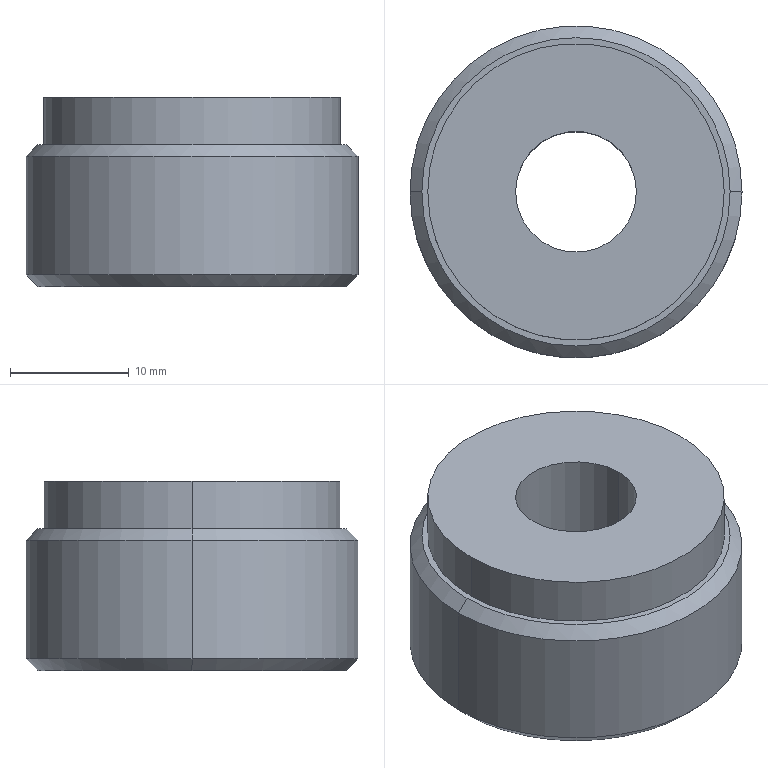Part | STEP file | Screen clamp lock nut 2 | 1 solid | 16 faces | box 28 x 28 x 16 mm | volume 7694 mm3 | cylinder 6 | cone 6 | plane 4 | commonest cylinder face diameters 10.2 x2 25 x2 28 x2
STEP:
#1=CARTESIAN_POINT('',(5.1,0.,1.));
#2=VERTEX_POINT('',#1);
#3=CARTESIAN_POINT('',(-5.1,0.,1.));
#4=VERTEX_POINT('',#3);
#5=CARTESIAN_POINT('',(0.,0.,1.));
#6=DIRECTION('',(0.,0.,-1.));
#7=DIRECTION('',(-1.,0.,0.));
#8=AXIS2_PLACEMENT_3D('',#5,#6,#7);
#9=CIRCLE('',#8,5.1);
#10=EDGE_CURVE('',#2,#4,#9,.T.);
#11=ORIENTED_EDGE('',*,*,#10,.T.);
#12=CARTESIAN_POINT('',(-5.1,0.,16.));
#13=VERTEX_POINT('',#12);
#14=CARTESIAN_POINT('',(-5.1,0.,16.));
#15=DIRECTION('',(0.,0.,1.));
#16=VECTOR('',#15,1000.);
#17=LINE('',#14,#16);
#18=EDGE_CURVE('',#4,#13,#17,.T.);
#19=ORIENTED_EDGE('',*,*,#18,.T.);
#20=CARTESIAN_POINT('',(5.1,0.,16.));
#21=VERTEX_POINT('',#20);
#22=CARTESIAN_POINT('',(0.,0.,16.));
#23=DIRECTION('',(0.,0.,1.));
#24=DIRECTION('',(1.,0.,0.));
#25=AXIS2_PLACEMENT_3D('',#22,#23,#24);
#26=CIRCLE('',#25,5.1);
#27=EDGE_CURVE('',#13,#21,#26,.T.);
#28=ORIENTED_EDGE('',*,*,#27,.T.);
#29=CARTESIAN_POINT('',(5.1,0.,16.));
#30=DIRECTION('',(0.,0.,1.));
#31=VECTOR('',#30,1000.);
#32=LINE('',#29,#31);
#33=EDGE_CURVE('',#2,#21,#32,.T.);
#34=ORIENTED_EDGE('',*,*,#33,.F.);
#35=EDGE_LOOP('',(#11,#19,#28,#34));
#36=FACE_OUTER_BOUND('',#35,.T.);
#37=CARTESIAN_POINT('',(0.,0.,16.));
#38=DIRECTION('',(0.,0.,1.));
#39=DIRECTION('',(1.,0.,0.));
#40=AXIS2_PLACEMENT_3D('',#37,#38,#39);
#41=CYLINDRICAL_SURFACE('',#40,5.1);
#42=ADVANCED_FACE('',(#36),#41,.F.);
#43=CARTESIAN_POINT('',(13.,0.,12.));
#44=VERTEX_POINT('',#43);
#45=CARTESIAN_POINT('',(-13.,0.,12.));
#46=VERTEX_POINT('',#45);
#47=CARTESIAN_POINT('',(0.,0.,12.));
#48=DIRECTION('',(0.,0.,1.));
#49=DIRECTION('',(1.,0.,0.));
#50=AXIS2_PLACEMENT_3D('',#47,#48,#49);
#51=CIRCLE('',#50,13.);
#52=EDGE_CURVE('',#44,#46,#51,.T.);
#53=ORIENTED_EDGE('',*,*,#52,.F.);
#54=CARTESIAN_POINT('',(14.,0.,11.));
#55=VERTEX_POINT('',#54);
#56=CARTESIAN_POINT('',(13.,0.,12.));
#57=DIRECTION('',(0.7071,0.,-0.7071));
#58=VECTOR('',#57,1000.);
#59=LINE('',#56,#58);
#60=EDGE_CURVE('',#44,#55,#59,.T.);
#61=ORIENTED_EDGE('',*,*,#60,.T.);
#62=CARTESIAN_POINT('',(-14.,0.,11.));
#63=VERTEX_POINT('',#62);
#64=CARTESIAN_POINT('',(0.,0.,11.));
#65=DIRECTION('',(0.,0.,-1.));
#66=DIRECTION('',(1.,0.,0.));
#67=AXIS2_PLACEMENT_3D('',#64,#65,#66);
#68=CIRCLE('',#67,14.);
#69=EDGE_CURVE('',#63,#55,#68,.T.);
#70=ORIENTED_EDGE('',*,*,#69,.F.);
#71=CARTESIAN_POINT('',(-13.,0.,12.));
#72=DIRECTION('',(-0.7071,0.,-0.7071));
#73=VECTOR('',#72,1000.);
#74=LINE('',#71,#73);
#75=EDGE_CURVE('',#46,#63,#74,.T.);
#76=ORIENTED_EDGE('',*,*,#75,.F.);
#77=EDGE_LOOP('',(#53,#61,#70,#76));
#78=FACE_OUTER_BOUND('',#77,.T.);
#79=CARTESIAN_POINT('',(0.,0.,12.));
#80=DIRECTION('',(0.,0.,-1.));
#81=DIRECTION('',(-1.,0.,0.));
#82=AXIS2_PLACEMENT_3D('',#79,#80,#81);
#83=CONICAL_SURFACE('',#82,13.,0.7854);
#84=ADVANCED_FACE('',(#78),#83,.T.);
#85=CARTESIAN_POINT('',(-13.,0.,0.));
#86=VERTEX_POINT('',#85);
#87=CARTESIAN_POINT('',(13.,0.,0.));
#88=VERTEX_POINT('',#87);
#89=CARTESIAN_POINT('',(0.,0.,0.));
#90=DIRECTION('',(0.,0.,-1.));
#91=DIRECTION('',(1.,0.,0.));
#92=AXIS2_PLACEMENT_3D('',#89,#90,#91);
#93=CIRCLE('',#92,13.);
#94=EDGE_CURVE('',#86,#88,#93,.T.);
#95=ORIENTED_EDGE('',*,*,#94,.F.);
#96=CARTESIAN_POINT('',(-14.,0.,1.));
#97=VERTEX_POINT('',#96);
#98=CARTESIAN_POINT('',(-14.,0.,1.));
#99=DIRECTION('',(-0.7071,0.,0.7071));
#100=VECTOR('',#99,1000.);
#101=LINE('',#98,#100);
#102=EDGE_CURVE('',#86,#97,#101,.T.);
#103=ORIENTED_EDGE('',*,*,#102,.T.);
#104=CARTESIAN_POINT('',(14.,0.,1.));
#105=VERTEX_POINT('',#104);
#106=CARTESIAN_POINT('',(0.,0.,1.));
#107=DIRECTION('',(0.,0.,1.));
#108=DIRECTION('',(1.,0.,0.));
#109=AXIS2_PLACEMENT_3D('',#106,#107,#108);
#110=CIRCLE('',#109,14.);
#111=EDGE_CURVE('',#105,#97,#110,.T.);
#112=ORIENTED_EDGE('',*,*,#111,.F.);
#113=CARTESIAN_POINT('',(14.,0.,1.));
#114=DIRECTION('',(0.7071,0.,0.7071));
#115=VECTOR('',#114,1000.);
#116=LINE('',#113,#115);
#117=EDGE_CURVE('',#88,#105,#116,.T.);
#118=ORIENTED_EDGE('',*,*,#117,.F.);
#119=EDGE_LOOP('',(#95,#103,#112,#118));
#120=FACE_OUTER_BOUND('',#119,.T.);
#121=CARTESIAN_POINT('',(0.,0.,1.));
#122=DIRECTION('',(0.,0.,1.));
#123=DIRECTION('',(1.,0.,0.));
#124=AXIS2_PLACEMENT_3D('',#121,#122,#123);
#125=CONICAL_SURFACE('',#124,14.,0.7854);
#126=ADVANCED_FACE('',(#120),#125,.T.);
#127=CARTESIAN_POINT('',(10.,0.,1.));
#128=VERTEX_POINT('',#127);
#129=CARTESIAN_POINT('',(-10.,0.,1.));
#130=VERTEX_POINT('',#129);
#131=CARTESIAN_POINT('',(0.,0.,1.));
#132=DIRECTION('',(0.,0.,-1.));
#133=DIRECTION('',(-1.,0.,0.));
#134=AXIS2_PLACEMENT_3D('',#131,#132,#133);
#135=CIRCLE('',#134,10.);
#136=EDGE_CURVE('',#128,#130,#135,.T.);
#137=ORIENTED_EDGE('',*,*,#136,.F.);
#138=CARTESIAN_POINT('',(11.,0.,0.));
#139=VERTEX_POINT('',#138);
#140=CARTESIAN_POINT('',(10.,0.,1.));
#141=DIRECTION('',(0.7071,0.,-0.7071));
#142=VECTOR('',#141,1000.);
#143=LINE('',#140,#142);
#144=EDGE_CURVE('',#128,#139,#143,.T.);
#145=ORIENTED_EDGE('',*,*,#144,.T.);
#146=CARTESIAN_POINT('',(-11.,0.,0.));
#147=VERTEX_POINT('',#146);
#148=CARTESIAN_POINT('',(0.,0.,0.));
#149=DIRECTION('',(0.,0.,1.));
#150=DIRECTION('',(1.,0.,0.));
#151=AXIS2_PLACEMENT_3D('',#148,#149,#150);
#152=CIRCLE('',#151,11.);
#153=EDGE_CURVE('',#147,#139,#152,.T.);
#154=ORIENTED_EDGE('',*,*,#153,.F.);
#155=CARTESIAN_POINT('',(-10.,0.,1.));
#156=DIRECTION('',(-0.7071,0.,-0.7071));
#157=VECTOR('',#156,1000.);
#158=LINE('',#155,#157);
#159=EDGE_CURVE('',#130,#147,#158,.T.);
#160=ORIENTED_EDGE('',*,*,#159,.F.);
#161=EDGE_LOOP('',(#137,#145,#154,#160));
#162=FACE_OUTER_BOUND('',#161,.T.);
#163=CARTESIAN_POINT('',(0.,0.,1.));
#164=DIRECTION('',(0.,0.,-1.));
#165=DIRECTION('',(-1.,0.,0.));
#166=AXIS2_PLACEMENT_3D('',#163,#164,#165);
#167=CONICAL_SURFACE('',#166,10.,0.7854);
#168=ADVANCED_FACE('',(#162),#167,.F.);
#169=CARTESIAN_POINT('',(12.5,0.,16.));
#170=VERTEX_POINT('',#169);
#171=CARTESIAN_POINT('',(-12.5,0.,16.));
#172=VERTEX_POINT('',#171);
#173=CARTESIAN_POINT('',(0.,0.,16.));
#174=DIRECTION('',(0.,0.,1.));
#175=DIRECTION('',(1.,0.,0.));
#176=AXIS2_PLACEMENT_3D('',#173,#174,#175);
#177=CIRCLE('',#176,12.5);
#178=EDGE_CURVE('',#170,#172,#177,.T.);
#179=ORIENTED_EDGE('',*,*,#178,.F.);
#180=CARTESIAN_POINT('',(12.5,0.,12.));
#181=VERTEX_POINT('',#180);
#182=CARTESIAN_POINT('',(12.5,0.,16.));
#183=DIRECTION('',(0.,0.,-1.));
#184=VECTOR('',#183,1000.);
#185=LINE('',#182,#184);
#186=EDGE_CURVE('',#170,#181,#185,.T.);
#187=ORIENTED_EDGE('',*,*,#186,.T.);
#188=CARTESIAN_POINT('',(-12.5,0.,12.));
#189=VERTEX_POINT('',#188);
#190=CARTESIAN_POINT('',(0.,0.,12.));
#191=DIRECTION('',(0.,0.,1.));
#192=DIRECTION('',(1.,0.,0.));
#193=AXIS2_PLACEMENT_3D('',#190,#191,#192);
#194=CIRCLE('',#193,12.5);
#195=EDGE_CURVE('',#181,#189,#194,.T.);
#196=ORIENTED_EDGE('',*,*,#195,.T.);
#197=CARTESIAN_POINT('',(-12.5,0.,16.));
#198=DIRECTION('',(0.,0.,-1.));
#199=VECTOR('',#198,1000.);
#200=LINE('',#197,#199);
#201=EDGE_CURVE('',#172,#189,#200,.T.);
#202=ORIENTED_EDGE('',*,*,#201,.F.);
#203=EDGE_LOOP('',(#179,#187,#196,#202));
#204=FACE_OUTER_BOUND('',#203,.T.);
#205=CARTESIAN_POINT('',(0.,0.,16.));
#206=DIRECTION('',(0.,0.,-1.));
#207=DIRECTION('',(-1.,0.,0.));
#208=AXIS2_PLACEMENT_3D('',#205,#206,#207);
#209=CYLINDRICAL_SURFACE('',#208,12.5);
#210=ADVANCED_FACE('',(#204),#209,.T.);
#211=ORIENTED_EDGE('',*,*,#69,.T.);
#212=CARTESIAN_POINT('',(14.,0.,12.));
#213=DIRECTION('',(0.,0.,-1.));
#214=VECTOR('',#213,1000.);
#215=LINE('',#212,#214);
#216=EDGE_CURVE('',#55,#105,#215,.T.);
#217=ORIENTED_EDGE('',*,*,#216,.T.);
#218=ORIENTED_EDGE('',*,*,#111,.T.);
#219=CARTESIAN_POINT('',(-14.,0.,12.));
#220=DIRECTION('',(0.,0.,-1.));
#221=VECTOR('',#220,1000.);
#222=LINE('',#219,#221);
#223=EDGE_CURVE('',#63,#97,#222,.T.);
#224=ORIENTED_EDGE('',*,*,#223,.F.);
#225=EDGE_LOOP('',(#211,#217,#218,#224));
#226=FACE_OUTER_BOUND('',#225,.T.);
#227=CARTESIAN_POINT('',(0.,0.,12.));
#228=DIRECTION('',(0.,0.,-1.));
#229=DIRECTION('',(-1.,0.,0.));
#230=AXIS2_PLACEMENT_3D('',#227,#228,#229);
#231=CYLINDRICAL_SURFACE('',#230,14.);
#232=ADVANCED_FACE('',(#226),#231,.T.);
#233=CARTESIAN_POINT('',(0.,0.,12.));
#234=DIRECTION('',(0.,0.,1.));
#235=DIRECTION('',(1.,0.,0.));
#236=AXIS2_PLACEMENT_3D('',#233,#234,#235);
#237=CIRCLE('',#236,13.);
#238=EDGE_CURVE('',#46,#44,#237,.T.);
#239=ORIENTED_EDGE('',*,*,#238,.T.);
#240=ORIENTED_EDGE('',*,*,#52,.T.);
#241=EDGE_LOOP('',(#239,#240));
#242=FACE_OUTER_BOUND('',#241,.T.);
#243=CARTESIAN_POINT('',(0.,0.,12.));
#244=DIRECTION('',(0.,0.,1.));
#245=DIRECTION('',(1.,0.,0.));
#246=AXIS2_PLACEMENT_3D('',#243,#244,#245);
#247=CIRCLE('',#246,12.5);
#248=EDGE_CURVE('',#189,#181,#247,.T.);
#249=ORIENTED_EDGE('',*,*,#248,.F.);
#250=ORIENTED_EDGE('',*,*,#195,.F.);
#251=EDGE_LOOP('',(#249,#250));
#252=FACE_BOUND('',#251,.T.);
#253=CARTESIAN_POINT('',(0.,0.,12.));
#254=DIRECTION('',(0.,0.,1.));
#255=DIRECTION('',(1.,0.,0.));
#256=AXIS2_PLACEMENT_3D('',#253,#254,#255);
#257=PLANE('',#256);
#258=ADVANCED_FACE('',(#242,#252),#257,.T.);
#259=ORIENTED_EDGE('',*,*,#216,.F.);
#260=CARTESIAN_POINT('',(0.,0.,11.));
#261=DIRECTION('',(0.,0.,-1.));
#262=DIRECTION('',(1.,0.,0.));
#263=AXIS2_PLACEMENT_3D('',#260,#261,#262);
#264=CIRCLE('',#263,14.);
#265=EDGE_CURVE('',#55,#63,#264,.T.);
#266=ORIENTED_EDGE('',*,*,#265,.T.);
#267=ORIENTED_EDGE('',*,*,#223,.T.);
#268=CARTESIAN_POINT('',(0.,0.,1.));
#269=DIRECTION('',(0.,0.,1.));
#270=DIRECTION('',(1.,0.,0.));
#271=AXIS2_PLACEMENT_3D('',#268,#269,#270);
#272=CIRCLE('',#271,14.);
#273=EDGE_CURVE('',#97,#105,#272,.T.);
#274=ORIENTED_EDGE('',*,*,#273,.T.);
#275=EDGE_LOOP('',(#259,#266,#267,#274));
#276=FACE_OUTER_BOUND('',#275,.T.);
#277=CARTESIAN_POINT('',(0.,0.,12.));
#278=DIRECTION('',(0.,0.,-1.));
#279=DIRECTION('',(-1.,0.,0.));
#280=AXIS2_PLACEMENT_3D('',#277,#278,#279);
#281=CYLINDRICAL_SURFACE('',#280,14.);
#282=ADVANCED_FACE('',(#276),#281,.T.);
#283=ORIENTED_EDGE('',*,*,#153,.T.);
#284=CARTESIAN_POINT('',(0.,0.,0.));
#285=DIRECTION('',(0.,0.,1.));
#286=DIRECTION('',(1.,0.,0.));
#287=AXIS2_PLACEMENT_3D('',#284,#285,#286);
#288=CIRCLE('',#287,11.);
#289=EDGE_CURVE('',#139,#147,#288,.T.);
#290=ORIENTED_EDGE('',*,*,#289,.T.);
#291=EDGE_LOOP('',(#283,#290));
#292=FACE_BOUND('',#291,.T.);
#293=CARTESIAN_POINT('',(0.,0.,0.));
#294=DIRECTION('',(0.,0.,-1.));
#295=DIRECTION('',(1.,0.,0.));
#296=AXIS2_PLACEMENT_3D('',#293,#294,#295);
#297=CIRCLE('',#296,13.);
#298=EDGE_CURVE('',#88,#86,#297,.T.);
#299=ORIENTED_EDGE('',*,*,#298,.T.);
#300=ORIENTED_EDGE('',*,*,#94,.T.);
#301=EDGE_LOOP('',(#299,#300));
#302=FACE_OUTER_BOUND('',#301,.T.);
#303=CARTESIAN_POINT('',(0.,0.,0.));
#304=DIRECTION('',(0.,0.,1.));
#305=DIRECTION('',(1.,0.,0.));
#306=AXIS2_PLACEMENT_3D('',#303,#304,#305);
#307=PLANE('',#306);
#308=ADVANCED_FACE('',(#292,#302),#307,.F.);
#309=ORIENTED_EDGE('',*,*,#186,.F.);
#310=CARTESIAN_POINT('',(0.,0.,16.));
#311=DIRECTION('',(0.,0.,1.));
#312=DIRECTION('',(1.,0.,0.));
#313=AXIS2_PLACEMENT_3D('',#310,#311,#312);
#314=CIRCLE('',#313,12.5);
#315=EDGE_CURVE('',#172,#170,#314,.T.);
#316=ORIENTED_EDGE('',*,*,#315,.F.);
#317=ORIENTED_EDGE('',*,*,#201,.T.);
#318=ORIENTED_EDGE('',*,*,#248,.T.);
#319=EDGE_LOOP('',(#309,#316,#317,#318));
#320=FACE_OUTER_BOUND('',#319,.T.);
#321=CARTESIAN_POINT('',(0.,0.,16.));
#322=DIRECTION('',(0.,0.,-1.));
#323=DIRECTION('',(-1.,0.,0.));
#324=AXIS2_PLACEMENT_3D('',#321,#322,#323);
#325=CYLINDRICAL_SURFACE('',#324,12.5);
#326=ADVANCED_FACE('',(#320),#325,.T.);
#327=CARTESIAN_POINT('',(0.,0.,16.));
#328=DIRECTION('',(0.,0.,1.));
#329=DIRECTION('',(1.,0.,0.));
#330=AXIS2_PLACEMENT_3D('',#327,#328,#329);
#331=CIRCLE('',#330,5.1);
#332=EDGE_CURVE('',#21,#13,#331,.T.);
#333=ORIENTED_EDGE('',*,*,#332,.F.);
#334=ORIENTED_EDGE('',*,*,#27,.F.);
#335=EDGE_LOOP('',(#333,#334));
#336=FACE_BOUND('',#335,.T.);
#337=ORIENTED_EDGE('',*,*,#315,.T.);
#338=ORIENTED_EDGE('',*,*,#178,.T.);
#339=EDGE_LOOP('',(#337,#338));
#340=FACE_OUTER_BOUND('',#339,.T.);
#341=CARTESIAN_POINT('',(0.,0.,16.));
#342=DIRECTION('',(0.,0.,1.));
#343=DIRECTION('',(1.,0.,0.));
#344=AXIS2_PLACEMENT_3D('',#341,#342,#343);
#345=PLANE('',#344);
#346=ADVANCED_FACE('',(#336,#340),#345,.T.);
#347=ORIENTED_EDGE('',*,*,#10,.F.);
#348=CARTESIAN_POINT('',(0.,0.,1.));
#349=DIRECTION('',(0.,0.,-1.));
#350=DIRECTION('',(-1.,0.,0.));
#351=AXIS2_PLACEMENT_3D('',#348,#349,#350);
#352=CIRCLE('',#351,5.1);
#353=EDGE_CURVE('',#4,#2,#352,.T.);
#354=ORIENTED_EDGE('',*,*,#353,.F.);
#355=EDGE_LOOP('',(#347,#354));
#356=FACE_BOUND('',#355,.T.);
#357=CARTESIAN_POINT('',(0.,0.,1.));
#358=DIRECTION('',(0.,0.,-1.));
#359=DIRECTION('',(-1.,0.,0.));
#360=AXIS2_PLACEMENT_3D('',#357,#358,#359);
#361=CIRCLE('',#360,10.);
#362=EDGE_CURVE('',#130,#128,#361,.T.);
#363=ORIENTED_EDGE('',*,*,#362,.T.);
#364=ORIENTED_EDGE('',*,*,#136,.T.);
#365=EDGE_LOOP('',(#363,#364));
#366=FACE_OUTER_BOUND('',#365,.T.);
#367=CARTESIAN_POINT('',(0.,0.,1.));
#368=DIRECTION('',(0.,0.,-1.));
#369=DIRECTION('',(-1.,0.,0.));
#370=AXIS2_PLACEMENT_3D('',#367,#368,#369);
#371=PLANE('',#370);
#372=ADVANCED_FACE('',(#356,#366),#371,.T.);
#373=ORIENTED_EDGE('',*,*,#144,.F.);
#374=ORIENTED_EDGE('',*,*,#362,.F.);
#375=ORIENTED_EDGE('',*,*,#159,.T.);
#376=ORIENTED_EDGE('',*,*,#289,.F.);
#377=EDGE_LOOP('',(#373,#374,#375,#376));
#378=FACE_OUTER_BOUND('',#377,.T.);
#379=CARTESIAN_POINT('',(0.,0.,1.));
#380=DIRECTION('',(0.,0.,-1.));
#381=DIRECTION('',(-1.,0.,0.));
#382=AXIS2_PLACEMENT_3D('',#379,#380,#381);
#383=CONICAL_SURFACE('',#382,10.,0.7854);
#384=ADVANCED_FACE('',(#378),#383,.F.);
#385=ORIENTED_EDGE('',*,*,#102,.F.);
#386=ORIENTED_EDGE('',*,*,#298,.F.);
#387=ORIENTED_EDGE('',*,*,#117,.T.);
#388=ORIENTED_EDGE('',*,*,#273,.F.);
#389=EDGE_LOOP('',(#385,#386,#387,#388));
#390=FACE_OUTER_BOUND('',#389,.T.);
#391=CARTESIAN_POINT('',(0.,0.,1.));
#392=DIRECTION('',(0.,0.,1.));
#393=DIRECTION('',(1.,0.,0.));
#394=AXIS2_PLACEMENT_3D('',#391,#392,#393);
#395=CONICAL_SURFACE('',#394,14.,0.7854);
#396=ADVANCED_FACE('',(#390),#395,.T.);
#397=ORIENTED_EDGE('',*,*,#60,.F.);
#398=ORIENTED_EDGE('',*,*,#238,.F.);
#399=ORIENTED_EDGE('',*,*,#75,.T.);
#400=ORIENTED_EDGE('',*,*,#265,.F.);
#401=EDGE_LOOP('',(#397,#398,#399,#400));
#402=FACE_OUTER_BOUND('',#401,.T.);
#403=CARTESIAN_POINT('',(0.,0.,12.));
#404=DIRECTION('',(0.,0.,-1.));
#405=DIRECTION('',(-1.,0.,0.));
#406=AXIS2_PLACEMENT_3D('',#403,#404,#405);
#407=CONICAL_SURFACE('',#406,13.,0.7854);
#408=ADVANCED_FACE('',(#402),#407,.T.);
#409=ORIENTED_EDGE('',*,*,#18,.F.);
#410=ORIENTED_EDGE('',*,*,#353,.T.);
#411=ORIENTED_EDGE('',*,*,#33,.T.);
#412=ORIENTED_EDGE('',*,*,#332,.T.);
#413=EDGE_LOOP('',(#409,#410,#411,#412));
#414=FACE_OUTER_BOUND('',#413,.T.);
#415=CARTESIAN_POINT('',(0.,0.,16.));
#416=DIRECTION('',(0.,0.,1.));
#417=DIRECTION('',(1.,0.,0.));
#418=AXIS2_PLACEMENT_3D('',#415,#416,#417);
#419=CYLINDRICAL_SURFACE('',#418,5.1);
#420=ADVANCED_FACE('',(#414),#419,.F.);
#421=CLOSED_SHELL('',(#42,#84,#126,#168,#210,#232,#258,#282,#308,#326,#346,#372,#384,#396,#408,#420));
#422=MANIFOLD_SOLID_BREP('',#421);
#423=CARTESIAN_POINT('',(0.,0.,0.));
#424=DIRECTION('',(0.,0.,1.));
#425=DIRECTION('',(1.,0.,0.));
#426=AXIS2_PLACEMENT_3D('',#423,#424,#425);
#427=(LENGTH_UNIT()NAMED_UNIT(*)SI_UNIT(.MILLI.,.METRE.));
#428=UNCERTAINTY_MEASURE_WITH_UNIT(LENGTH_MEASURE(0.00001),#427,'','');
#429=(NAMED_UNIT(*)PLANE_ANGLE_UNIT()SI_UNIT($,.RADIAN.));
#430=(NAMED_UNIT(*)SI_UNIT($,.STERADIAN.)SOLID_ANGLE_UNIT());
#431=(GEOMETRIC_REPRESENTATION_CONTEXT(3)GLOBAL_UNCERTAINTY_ASSIGNED_CONTEXT((#428))GLOBAL_UNIT_ASSIGNED_CONTEXT((#427,#429,#430))REPRESENTATION_CONTEXT('',''));
#432=ADVANCED_BREP_SHAPE_REPRESENTATION('',(#422,#426),#431);